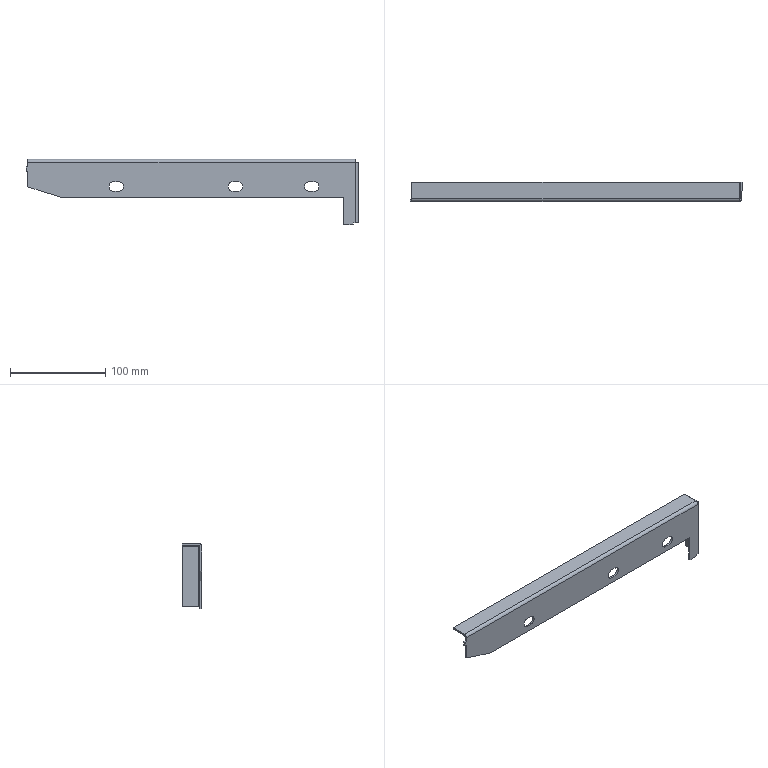Part | 1 solid | 43 faces | box 348 x 20 x 68.5 mm | volume 41297 mm3 | plane 33 | cylinder 10 | commonest cylinder face diameters 10 x6 2 x2 6 x2
STEP:
#1=CARTESIAN_POINT('',(-343.,-2.,53.5));
#2=VERTEX_POINT('',#1);
#3=CARTESIAN_POINT('',(-343.,-2.,37.5));
#4=VERTEX_POINT('',#3);
#5=CARTESIAN_POINT('',(-343.,-2.,63.5));
#6=DIRECTION('',(0.,0.,-1.));
#7=VECTOR('',#6,1000.);
#8=LINE('',#5,#7);
#9=EDGE_CURVE('',#2,#4,#8,.T.);
#10=ORIENTED_EDGE('',*,*,#9,.F.);
#11=CARTESIAN_POINT('',(-343.,0.,53.5));
#12=VERTEX_POINT('',#11);
#13=CARTESIAN_POINT('',(-343.,0.,53.5));
#14=DIRECTION('',(0.,-1.,0.));
#15=VECTOR('',#14,1000.);
#16=LINE('',#13,#15);
#17=EDGE_CURVE('',#12,#2,#16,.T.);
#18=ORIENTED_EDGE('',*,*,#17,.F.);
#19=CARTESIAN_POINT('',(-343.,0.,37.5));
#20=VERTEX_POINT('',#19);
#21=CARTESIAN_POINT('',(-343.,0.,63.5));
#22=DIRECTION('',(0.,0.,-1.));
#23=VECTOR('',#22,1000.);
#24=LINE('',#21,#23);
#25=EDGE_CURVE('',#12,#20,#24,.T.);
#26=ORIENTED_EDGE('',*,*,#25,.T.);
#27=CARTESIAN_POINT('',(-343.,8.,37.5));
#28=DIRECTION('',(0.,-1.,0.));
#29=VECTOR('',#28,1000.);
#30=LINE('',#27,#29);
#31=EDGE_CURVE('',#20,#4,#30,.T.);
#32=ORIENTED_EDGE('',*,*,#31,.T.);
#33=EDGE_LOOP('',(#10,#18,#26,#32));
#34=FACE_OUTER_BOUND('',#33,.T.);
#35=CARTESIAN_POINT('',(-343.,-2.,63.5));
#36=DIRECTION('',(-1.,0.,0.));
#37=DIRECTION('',(0.,0.,1.));
#38=AXIS2_PLACEMENT_3D('',#35,#36,#37);
#39=PLANE('',#38);
#40=ADVANCED_FACE('',(#34),#39,.T.);
#41=CARTESIAN_POINT('',(-343.,0.,63.5));
#42=VERTEX_POINT('',#41);
#43=CARTESIAN_POINT('',(-343.,0.,58.5));
#44=VERTEX_POINT('',#43);
#45=CARTESIAN_POINT('',(-343.,0.,63.5));
#46=DIRECTION('',(0.,0.,-1.));
#47=VECTOR('',#46,1000.);
#48=LINE('',#45,#47);
#49=EDGE_CURVE('',#42,#44,#48,.T.);
#50=ORIENTED_EDGE('',*,*,#49,.T.);
#51=CARTESIAN_POINT('',(-343.,-2.,58.5));
#52=VERTEX_POINT('',#51);
#53=CARTESIAN_POINT('',(-343.,0.,58.5));
#54=DIRECTION('',(0.,1.,0.));
#55=VECTOR('',#54,1000.);
#56=LINE('',#53,#55);
#57=EDGE_CURVE('',#52,#44,#56,.T.);
#58=ORIENTED_EDGE('',*,*,#57,.F.);
#59=CARTESIAN_POINT('',(-343.,-2.,63.5));
#60=VERTEX_POINT('',#59);
#61=CARTESIAN_POINT('',(-343.,-2.,63.5));
#62=DIRECTION('',(0.,0.,-1.));
#63=VECTOR('',#62,1000.);
#64=LINE('',#61,#63);
#65=EDGE_CURVE('',#60,#52,#64,.T.);
#66=ORIENTED_EDGE('',*,*,#65,.F.);
#67=CARTESIAN_POINT('',(-343.,-2.,63.5));
#68=DIRECTION('',(0.,1.,0.));
#69=VECTOR('',#68,1000.);
#70=LINE('',#67,#69);
#71=EDGE_CURVE('',#60,#42,#70,.T.);
#72=ORIENTED_EDGE('',*,*,#71,.T.);
#73=EDGE_LOOP('',(#50,#58,#66,#72));
#74=FACE_OUTER_BOUND('',#73,.T.);
#75=CARTESIAN_POINT('',(-343.,-2.,63.5));
#76=DIRECTION('',(-1.,0.,0.));
#77=DIRECTION('',(0.,0.,1.));
#78=AXIS2_PLACEMENT_3D('',#75,#76,#77);
#79=PLANE('',#78);
#80=ADVANCED_FACE('',(#74),#79,.T.);
#81=CARTESIAN_POINT('',(-253.,-2.,33.));
#82=VERTEX_POINT('',#81);
#83=CARTESIAN_POINT('',(-248.,-2.,33.));
#84=VERTEX_POINT('',#83);
#85=CARTESIAN_POINT('',(-253.,-2.,33.));
#86=DIRECTION('',(1.,0.,0.));
#87=VECTOR('',#86,1000.);
#88=LINE('',#85,#87);
#89=EDGE_CURVE('',#82,#84,#88,.T.);
#90=ORIENTED_EDGE('',*,*,#89,.F.);
#91=CARTESIAN_POINT('',(-253.,-2.,43.));
#92=VERTEX_POINT('',#91);
#93=CARTESIAN_POINT('',(-253.,-2.,38.));
#94=DIRECTION('',(0.,-1.,0.));
#95=DIRECTION('',(0.,0.,-1.));
#96=AXIS2_PLACEMENT_3D('',#93,#94,#95);
#97=CIRCLE('',#96,5.);
#98=EDGE_CURVE('',#92,#82,#97,.T.);
#99=ORIENTED_EDGE('',*,*,#98,.F.);
#100=CARTESIAN_POINT('',(-248.,-2.,43.));
#101=VERTEX_POINT('',#100);
#102=CARTESIAN_POINT('',(-253.,-2.,43.));
#103=DIRECTION('',(-1.,0.,0.));
#104=VECTOR('',#103,1000.);
#105=LINE('',#102,#104);
#106=EDGE_CURVE('',#101,#92,#105,.T.);
#107=ORIENTED_EDGE('',*,*,#106,.F.);
#108=CARTESIAN_POINT('',(-248.,-2.,38.));
#109=DIRECTION('',(0.,-1.,0.));
#110=DIRECTION('',(0.,0.,-1.));
#111=AXIS2_PLACEMENT_3D('',#108,#109,#110);
#112=CIRCLE('',#111,5.);
#113=EDGE_CURVE('',#84,#101,#112,.T.);
#114=ORIENTED_EDGE('',*,*,#113,.F.);
#115=EDGE_LOOP('',(#90,#99,#107,#114));
#116=FACE_BOUND('',#115,.T.);
#117=CARTESIAN_POINT('',(-128.,-2.,33.));
#118=VERTEX_POINT('',#117);
#119=CARTESIAN_POINT('',(-123.,-2.,33.));
#120=VERTEX_POINT('',#119);
#121=CARTESIAN_POINT('',(-128.,-2.,33.));
#122=DIRECTION('',(1.,0.,0.));
#123=VECTOR('',#122,1000.);
#124=LINE('',#121,#123);
#125=EDGE_CURVE('',#118,#120,#124,.T.);
#126=ORIENTED_EDGE('',*,*,#125,.F.);
#127=CARTESIAN_POINT('',(-128.,-2.,43.));
#128=VERTEX_POINT('',#127);
#129=CARTESIAN_POINT('',(-128.,-2.,38.));
#130=DIRECTION('',(0.,-1.,0.));
#131=DIRECTION('',(0.,0.,-1.));
#132=AXIS2_PLACEMENT_3D('',#129,#130,#131);
#133=CIRCLE('',#132,5.);
#134=EDGE_CURVE('',#128,#118,#133,.T.);
#135=ORIENTED_EDGE('',*,*,#134,.F.);
#136=CARTESIAN_POINT('',(-123.,-2.,43.));
#137=VERTEX_POINT('',#136);
#138=CARTESIAN_POINT('',(-128.,-2.,43.));
#139=DIRECTION('',(-1.,0.,0.));
#140=VECTOR('',#139,1000.);
#141=LINE('',#138,#140);
#142=EDGE_CURVE('',#137,#128,#141,.T.);
#143=ORIENTED_EDGE('',*,*,#142,.F.);
#144=CARTESIAN_POINT('',(-123.,-2.,38.));
#145=DIRECTION('',(0.,-1.,0.));
#146=DIRECTION('',(0.,0.,-1.));
#147=AXIS2_PLACEMENT_3D('',#144,#145,#146);
#148=CIRCLE('',#147,5.);
#149=EDGE_CURVE('',#120,#137,#148,.T.);
#150=ORIENTED_EDGE('',*,*,#149,.F.);
#151=EDGE_LOOP('',(#126,#135,#143,#150));
#152=FACE_BOUND('',#151,.T.);
#153=CARTESIAN_POINT('',(-48.,-2.,33.));
#154=VERTEX_POINT('',#153);
#155=CARTESIAN_POINT('',(-43.,-2.,33.));
#156=VERTEX_POINT('',#155);
#157=CARTESIAN_POINT('',(-48.,-2.,33.));
#158=DIRECTION('',(1.,0.,0.));
#159=VECTOR('',#158,1000.);
#160=LINE('',#157,#159);
#161=EDGE_CURVE('',#154,#156,#160,.T.);
#162=ORIENTED_EDGE('',*,*,#161,.F.);
#163=CARTESIAN_POINT('',(-48.,-2.,43.));
#164=VERTEX_POINT('',#163);
#165=CARTESIAN_POINT('',(-48.,-2.,38.));
#166=DIRECTION('',(0.,-1.,0.));
#167=DIRECTION('',(0.,0.,-1.));
#168=AXIS2_PLACEMENT_3D('',#165,#166,#167);
#169=CIRCLE('',#168,5.);
#170=EDGE_CURVE('',#164,#154,#169,.T.);
#171=ORIENTED_EDGE('',*,*,#170,.F.);
#172=CARTESIAN_POINT('',(-43.,-2.,43.));
#173=VERTEX_POINT('',#172);
#174=CARTESIAN_POINT('',(-48.,-2.,43.));
#175=DIRECTION('',(-1.,0.,0.));
#176=VECTOR('',#175,1000.);
#177=LINE('',#174,#176);
#178=EDGE_CURVE('',#173,#164,#177,.T.);
#179=ORIENTED_EDGE('',*,*,#178,.F.);
#180=CARTESIAN_POINT('',(-43.,-2.,38.));
#181=DIRECTION('',(0.,-1.,0.));
#182=DIRECTION('',(0.,0.,-1.));
#183=AXIS2_PLACEMENT_3D('',#180,#181,#182);
#184=CIRCLE('',#183,5.);
#185=EDGE_CURVE('',#156,#173,#184,.T.);
#186=ORIENTED_EDGE('',*,*,#185,.F.);
#187=EDGE_LOOP('',(#162,#171,#179,#186));
#188=FACE_BOUND('',#187,.T.);
#189=ORIENTED_EDGE('',*,*,#65,.T.);
#190=CARTESIAN_POINT('',(-345.,-2.,58.5));
#191=VERTEX_POINT('',#190);
#192=CARTESIAN_POINT('',(-345.,-2.,58.5));
#193=DIRECTION('',(1.,0.,0.));
#194=VECTOR('',#193,1000.);
#195=LINE('',#192,#194);
#196=EDGE_CURVE('',#191,#52,#195,.T.);
#197=ORIENTED_EDGE('',*,*,#196,.F.);
#198=CARTESIAN_POINT('',(-345.,-2.,53.5));
#199=VERTEX_POINT('',#198);
#200=CARTESIAN_POINT('',(-345.,-2.,53.5));
#201=DIRECTION('',(0.,0.,1.));
#202=VECTOR('',#201,1000.);
#203=LINE('',#200,#202);
#204=EDGE_CURVE('',#199,#191,#203,.T.);
#205=ORIENTED_EDGE('',*,*,#204,.F.);
#206=CARTESIAN_POINT('',(-345.,-2.,53.5));
#207=DIRECTION('',(1.,0.,0.));
#208=VECTOR('',#207,1000.);
#209=LINE('',#206,#208);
#210=EDGE_CURVE('',#199,#2,#209,.T.);
#211=ORIENTED_EDGE('',*,*,#210,.T.);
#212=ORIENTED_EDGE('',*,*,#9,.T.);
#213=CARTESIAN_POINT('',(-308.,-2.,26.5));
#214=VERTEX_POINT('',#213);
#215=CARTESIAN_POINT('',(-343.,-2.,37.5));
#216=DIRECTION('',(-0.954,0.,0.2998));
#217=VECTOR('',#216,1000.);
#218=LINE('',#215,#217);
#219=EDGE_CURVE('',#214,#4,#218,.T.);
#220=ORIENTED_EDGE('',*,*,#219,.F.);
#221=CARTESIAN_POINT('',(-12.,-2.,26.5));
#222=VERTEX_POINT('',#221);
#223=CARTESIAN_POINT('',(-343.,-2.,26.5));
#224=DIRECTION('',(-1.,0.,0.));
#225=VECTOR('',#224,1000.);
#226=LINE('',#223,#225);
#227=EDGE_CURVE('',#222,#214,#226,.T.);
#228=ORIENTED_EDGE('',*,*,#227,.F.);
#229=CARTESIAN_POINT('',(-12.,-2.,-2.));
#230=VERTEX_POINT('',#229);
#231=CARTESIAN_POINT('',(-12.,-2.,0.));
#232=DIRECTION('',(0.,0.,1.));
#233=VECTOR('',#232,1000.);
#234=LINE('',#231,#233);
#235=EDGE_CURVE('',#230,#222,#234,.T.);
#236=ORIENTED_EDGE('',*,*,#235,.F.);
#237=CARTESIAN_POINT('',(-2.,-2.,-2.));
#238=VERTEX_POINT('',#237);
#239=CARTESIAN_POINT('',(-12.,-2.,-2.));
#240=DIRECTION('',(1.,0.,0.));
#241=VECTOR('',#240,1000.);
#242=LINE('',#239,#241);
#243=EDGE_CURVE('',#230,#238,#242,.T.);
#244=ORIENTED_EDGE('',*,*,#243,.T.);
#245=CARTESIAN_POINT('',(-2.,-2.,0.));
#246=VERTEX_POINT('',#245);
#247=CARTESIAN_POINT('',(-2.,-2.,0.));
#248=DIRECTION('',(0.,0.,1.));
#249=VECTOR('',#248,1000.);
#250=LINE('',#247,#249);
#251=EDGE_CURVE('',#238,#246,#250,.T.);
#252=ORIENTED_EDGE('',*,*,#251,.T.);
#253=CARTESIAN_POINT('',(0.,-2.,0.));
#254=VERTEX_POINT('',#253);
#255=CARTESIAN_POINT('',(-343.,-2.,0.));
#256=DIRECTION('',(1.,0.,0.));
#257=VECTOR('',#256,1000.);
#258=LINE('',#255,#257);
#259=EDGE_CURVE('',#246,#254,#258,.T.);
#260=ORIENTED_EDGE('',*,*,#259,.T.);
#261=CARTESIAN_POINT('',(0.,-2.,63.5));
#262=VERTEX_POINT('',#261);
#263=CARTESIAN_POINT('',(0.,-2.,63.5));
#264=DIRECTION('',(0.,0.,-1.));
#265=VECTOR('',#264,1000.);
#266=LINE('',#263,#265);
#267=EDGE_CURVE('',#262,#254,#266,.T.);
#268=ORIENTED_EDGE('',*,*,#267,.F.);
#269=CARTESIAN_POINT('',(-343.,-2.,63.5));
#270=DIRECTION('',(1.,0.,0.));
#271=VECTOR('',#270,1000.);
#272=LINE('',#269,#271);
#273=EDGE_CURVE('',#60,#262,#272,.T.);
#274=ORIENTED_EDGE('',*,*,#273,.F.);
#275=EDGE_LOOP('',(#189,#197,#205,#211,#212,#220,#228,#236,#244,#252,#260,#268,#274));
#276=FACE_OUTER_BOUND('',#275,.T.);
#277=CARTESIAN_POINT('',(-343.,-2.,63.5));
#278=DIRECTION('',(0.,1.,0.));
#279=DIRECTION('',(0.,0.,1.));
#280=AXIS2_PLACEMENT_3D('',#277,#278,#279);
#281=PLANE('',#280);
#282=ADVANCED_FACE('',(#116,#152,#188,#276),#281,.F.);
#283=CARTESIAN_POINT('',(-308.,0.,26.5));
#284=VERTEX_POINT('',#283);
#285=CARTESIAN_POINT('',(-350.437,0.,39.837));
#286=DIRECTION('',(0.954,0.,-0.2998));
#287=VECTOR('',#286,1000.);
#288=LINE('',#285,#287);
#289=EDGE_CURVE('',#20,#284,#288,.T.);
#290=ORIENTED_EDGE('',*,*,#289,.F.);
#291=ORIENTED_EDGE('',*,*,#25,.F.);
#292=CARTESIAN_POINT('',(-345.,0.,53.5));
#293=VERTEX_POINT('',#292);
#294=CARTESIAN_POINT('',(-345.,0.,53.5));
#295=DIRECTION('',(1.,0.,0.));
#296=VECTOR('',#295,1000.);
#297=LINE('',#294,#296);
#298=EDGE_CURVE('',#293,#12,#297,.T.);
#299=ORIENTED_EDGE('',*,*,#298,.F.);
#300=CARTESIAN_POINT('',(-345.,0.,58.5));
#301=VERTEX_POINT('',#300);
#302=CARTESIAN_POINT('',(-345.,0.,53.5));
#303=DIRECTION('',(0.,0.,-1.));
#304=VECTOR('',#303,1000.);
#305=LINE('',#302,#304);
#306=EDGE_CURVE('',#301,#293,#305,.T.);
#307=ORIENTED_EDGE('',*,*,#306,.F.);
#308=CARTESIAN_POINT('',(-345.,0.,58.5));
#309=DIRECTION('',(1.,0.,0.));
#310=VECTOR('',#309,1000.);
#311=LINE('',#308,#310);
#312=EDGE_CURVE('',#301,#44,#311,.T.);
#313=ORIENTED_EDGE('',*,*,#312,.T.);
#314=ORIENTED_EDGE('',*,*,#49,.F.);
#315=CARTESIAN_POINT('',(0.,0.,63.5));
#316=VERTEX_POINT('',#315);
#317=CARTESIAN_POINT('',(-343.,0.,63.5));
#318=DIRECTION('',(1.,0.,0.));
#319=VECTOR('',#318,1000.);
#320=LINE('',#317,#319);
#321=EDGE_CURVE('',#42,#316,#320,.T.);
#322=ORIENTED_EDGE('',*,*,#321,.T.);
#323=CARTESIAN_POINT('',(0.,0.,0.));
#324=VERTEX_POINT('',#323);
#325=CARTESIAN_POINT('',(0.,0.,63.5));
#326=DIRECTION('',(0.,0.,-1.));
#327=VECTOR('',#326,1000.);
#328=LINE('',#325,#327);
#329=EDGE_CURVE('',#316,#324,#328,.T.);
#330=ORIENTED_EDGE('',*,*,#329,.T.);
#331=CARTESIAN_POINT('',(-2.,0.,0.));
#332=VERTEX_POINT('',#331);
#333=CARTESIAN_POINT('',(-343.,0.,0.));
#334=DIRECTION('',(1.,0.,0.));
#335=VECTOR('',#334,1000.);
#336=LINE('',#333,#335);
#337=EDGE_CURVE('',#332,#324,#336,.T.);
#338=ORIENTED_EDGE('',*,*,#337,.F.);
#339=CARTESIAN_POINT('',(-2.,0.,-2.));
#340=VERTEX_POINT('',#339);
#341=CARTESIAN_POINT('',(-2.,0.,0.));
#342=DIRECTION('',(0.,0.,1.));
#343=VECTOR('',#342,1000.);
#344=LINE('',#341,#343);
#345=EDGE_CURVE('',#340,#332,#344,.T.);
#346=ORIENTED_EDGE('',*,*,#345,.F.);
#347=CARTESIAN_POINT('',(-12.,0.,-2.));
#348=VERTEX_POINT('',#347);
#349=CARTESIAN_POINT('',(-12.,0.,-2.));
#350=DIRECTION('',(1.,0.,0.));
#351=VECTOR('',#350,1000.);
#352=LINE('',#349,#351);
#353=EDGE_CURVE('',#348,#340,#352,.T.);
#354=ORIENTED_EDGE('',*,*,#353,.F.);
#355=CARTESIAN_POINT('',(-12.,0.,26.5));
#356=VERTEX_POINT('',#355);
#357=CARTESIAN_POINT('',(-12.,0.,63.5));
#358=DIRECTION('',(0.,0.,-1.));
#359=VECTOR('',#358,1000.);
#360=LINE('',#357,#359);
#361=EDGE_CURVE('',#356,#348,#360,.T.);
#362=ORIENTED_EDGE('',*,*,#361,.F.);
#363=CARTESIAN_POINT('',(-343.,0.,26.5));
#364=DIRECTION('',(1.,0.,0.));
#365=VECTOR('',#364,1000.);
#366=LINE('',#363,#365);
#367=EDGE_CURVE('',#284,#356,#366,.T.);
#368=ORIENTED_EDGE('',*,*,#367,.F.);
#369=EDGE_LOOP('',(#290,#291,#299,#307,#313,#314,#322,#330,#338,#346,#354,#362,#368));
#370=FACE_OUTER_BOUND('',#369,.T.);
#371=CARTESIAN_POINT('',(-253.,0.,33.));
#372=VERTEX_POINT('',#371);
#373=CARTESIAN_POINT('',(-253.,0.,43.));
#374=VERTEX_POINT('',#373);
#375=CARTESIAN_POINT('',(-253.,0.,38.));
#376=DIRECTION('',(0.,1.,0.));
#377=DIRECTION('',(0.,0.,1.));
#378=AXIS2_PLACEMENT_3D('',#375,#376,#377);
#379=CIRCLE('',#378,5.);
#380=EDGE_CURVE('',#372,#374,#379,.T.);
#381=ORIENTED_EDGE('',*,*,#380,.F.);
#382=CARTESIAN_POINT('',(-248.,0.,33.));
#383=VERTEX_POINT('',#382);
#384=CARTESIAN_POINT('',(-343.,0.,33.));
#385=DIRECTION('',(-1.,0.,0.));
#386=VECTOR('',#385,1000.);
#387=LINE('',#384,#386);
#388=EDGE_CURVE('',#383,#372,#387,.T.);
#389=ORIENTED_EDGE('',*,*,#388,.F.);
#390=CARTESIAN_POINT('',(-248.,0.,43.));
#391=VERTEX_POINT('',#390);
#392=CARTESIAN_POINT('',(-248.,0.,38.));
#393=DIRECTION('',(0.,1.,0.));
#394=DIRECTION('',(0.,0.,1.));
#395=AXIS2_PLACEMENT_3D('',#392,#393,#394);
#396=CIRCLE('',#395,5.);
#397=EDGE_CURVE('',#391,#383,#396,.T.);
#398=ORIENTED_EDGE('',*,*,#397,.F.);
#399=CARTESIAN_POINT('',(-343.,0.,43.));
#400=DIRECTION('',(1.,0.,0.));
#401=VECTOR('',#400,1000.);
#402=LINE('',#399,#401);
#403=EDGE_CURVE('',#374,#391,#402,.T.);
#404=ORIENTED_EDGE('',*,*,#403,.F.);
#405=EDGE_LOOP('',(#381,#389,#398,#404));
#406=FACE_BOUND('',#405,.T.);
#407=CARTESIAN_POINT('',(-128.,0.,33.));
#408=VERTEX_POINT('',#407);
#409=CARTESIAN_POINT('',(-128.,0.,43.));
#410=VERTEX_POINT('',#409);
#411=CARTESIAN_POINT('',(-128.,0.,38.));
#412=DIRECTION('',(0.,1.,0.));
#413=DIRECTION('',(0.,0.,1.));
#414=AXIS2_PLACEMENT_3D('',#411,#412,#413);
#415=CIRCLE('',#414,5.);
#416=EDGE_CURVE('',#408,#410,#415,.T.);
#417=ORIENTED_EDGE('',*,*,#416,.F.);
#418=CARTESIAN_POINT('',(-123.,0.,33.));
#419=VERTEX_POINT('',#418);
#420=CARTESIAN_POINT('',(-343.,0.,33.));
#421=DIRECTION('',(-1.,0.,0.));
#422=VECTOR('',#421,1000.);
#423=LINE('',#420,#422);
#424=EDGE_CURVE('',#419,#408,#423,.T.);
#425=ORIENTED_EDGE('',*,*,#424,.F.);
#426=CARTESIAN_POINT('',(-123.,0.,43.));
#427=VERTEX_POINT('',#426);
#428=CARTESIAN_POINT('',(-123.,0.,38.));
#429=DIRECTION('',(0.,1.,0.));
#430=DIRECTION('',(0.,0.,1.));
#431=AXIS2_PLACEMENT_3D('',#428,#429,#430);
#432=CIRCLE('',#431,5.);
#433=EDGE_CURVE('',#427,#419,#432,.T.);
#434=ORIENTED_EDGE('',*,*,#433,.F.);
#435=CARTESIAN_POINT('',(-343.,0.,43.));
#436=DIRECTION('',(1.,0.,0.));
#437=VECTOR('',#436,1000.);
#438=LINE('',#435,#437);
#439=EDGE_CURVE('',#410,#427,#438,.T.);
#440=ORIENTED_EDGE('',*,*,#439,.F.);
#441=EDGE_LOOP('',(#417,#425,#434,#440));
#442=FACE_BOUND('',#441,.T.);
#443=CARTESIAN_POINT('',(-48.,0.,33.));
#444=VERTEX_POINT('',#443);
#445=CARTESIAN_POINT('',(-48.,0.,43.));
#446=VERTEX_POINT('',#445);
#447=CARTESIAN_POINT('',(-48.,0.,38.));
#448=DIRECTION('',(0.,1.,0.));
#449=DIRECTION('',(0.,0.,1.));
#450=AXIS2_PLACEMENT_3D('',#447,#448,#449);
#451=CIRCLE('',#450,5.);
#452=EDGE_CURVE('',#444,#446,#451,.T.);
#453=ORIENTED_EDGE('',*,*,#452,.F.);
#454=CARTESIAN_POINT('',(-43.,0.,33.));
#455=VERTEX_POINT('',#454);
#456=CARTESIAN_POINT('',(-343.,0.,33.));
#457=DIRECTION('',(-1.,0.,0.));
#458=VECTOR('',#457,1000.);
#459=LINE('',#456,#458);
#460=EDGE_CURVE('',#455,#444,#459,.T.);
#461=ORIENTED_EDGE('',*,*,#460,.F.);
#462=CARTESIAN_POINT('',(-43.,0.,43.));
#463=VERTEX_POINT('',#462);
#464=CARTESIAN_POINT('',(-43.,0.,38.));
#465=DIRECTION('',(0.,1.,0.));
#466=DIRECTION('',(0.,0.,1.));
#467=AXIS2_PLACEMENT_3D('',#464,#465,#466);
#468=CIRCLE('',#467,5.);
#469=EDGE_CURVE('',#463,#455,#468,.T.);
#470=ORIENTED_EDGE('',*,*,#469,.F.);
#471=CARTESIAN_POINT('',(-343.,0.,43.));
#472=DIRECTION('',(1.,0.,0.));
#473=VECTOR('',#472,1000.);
#474=LINE('',#471,#473);
#475=EDGE_CURVE('',#446,#463,#474,.T.);
#476=ORIENTED_EDGE('',*,*,#475,.F.);
#477=EDGE_LOOP('',(#453,#461,#470,#476));
#478=FACE_BOUND('',#477,.T.);
#479=CARTESIAN_POINT('',(-343.,0.,63.5));
#480=DIRECTION('',(0.,1.,0.));
#481=DIRECTION('',(0.,0.,1.));
#482=AXIS2_PLACEMENT_3D('',#479,#480,#481);
#483=PLANE('',#482);
#484=ADVANCED_FACE('',(#370,#406,#442,#478),#483,.T.);
#485=CARTESIAN_POINT('',(-2.,0.,0.));
#486=DIRECTION('',(0.,-1.,0.));
#487=VECTOR('',#486,1000.);
#488=LINE('',#485,#487);
#489=EDGE_CURVE('',#332,#246,#488,.T.);
#490=ORIENTED_EDGE('',*,*,#489,.F.);
#491=ORIENTED_EDGE('',*,*,#337,.T.);
#492=CARTESIAN_POINT('',(0.,0.,0.));
#493=DIRECTION('',(0.,-1.,0.));
#494=VECTOR('',#493,1000.);
#495=LINE('',#492,#494);
#496=EDGE_CURVE('',#324,#254,#495,.T.);
#497=ORIENTED_EDGE('',*,*,#496,.T.);
#498=ORIENTED_EDGE('',*,*,#259,.F.);
#499=EDGE_LOOP('',(#490,#491,#497,#498));
#500=FACE_OUTER_BOUND('',#499,.T.);
#501=CARTESIAN_POINT('',(0.,0.,0.));
#502=DIRECTION('',(0.,0.,-1.));
#503=DIRECTION('',(-1.,0.,0.));
#504=AXIS2_PLACEMENT_3D('',#501,#502,#503);
#505=PLANE('',#504);
#506=ADVANCED_FACE('',(#500),#505,.T.);
#507=CARTESIAN_POINT('',(-343.,1.,64.5));
#508=VERTEX_POINT('',#507);
#509=CARTESIAN_POINT('',(-343.,1.,66.5));
#510=VERTEX_POINT('',#509);
#511=CARTESIAN_POINT('',(-343.,1.,66.5));
#512=DIRECTION('',(0.,0.,1.));
#513=VECTOR('',#512,1000.);
#514=LINE('',#511,#513);
#515=EDGE_CURVE('',#508,#510,#514,.T.);
#516=ORIENTED_EDGE('',*,*,#515,.F.);
#517=CARTESIAN_POINT('',(-343.,1.,63.5));
#518=DIRECTION('',(-1.,0.,0.));
#519=DIRECTION('',(0.,0.,-1.));
#520=AXIS2_PLACEMENT_3D('',#517,#518,#519);
#521=CIRCLE('',#520,1.);
#522=EDGE_CURVE('',#42,#508,#521,.T.);
#523=ORIENTED_EDGE('',*,*,#522,.F.);
#524=ORIENTED_EDGE('',*,*,#71,.F.);
#525=CARTESIAN_POINT('',(-343.,1.,63.5));
#526=DIRECTION('',(-1.,0.,0.));
#527=DIRECTION('',(0.,0.,-1.));
#528=AXIS2_PLACEMENT_3D('',#525,#526,#527);
#529=CIRCLE('',#528,3.);
#530=EDGE_CURVE('',#60,#510,#529,.T.);
#531=ORIENTED_EDGE('',*,*,#530,.T.);
#532=EDGE_LOOP('',(#516,#523,#524,#531));
#533=FACE_OUTER_BOUND('',#532,.T.);
#534=CARTESIAN_POINT('',(-343.,1.,63.5));
#535=DIRECTION('',(-1.,0.,0.));
#536=DIRECTION('',(0.,0.,1.));
#537=AXIS2_PLACEMENT_3D('',#534,#535,#536);
#538=PLANE('',#537);
#539=ADVANCED_FACE('',(#533),#538,.T.);
#540=CARTESIAN_POINT('',(0.,1.,64.5));
#541=VERTEX_POINT('',#540);
#542=CARTESIAN_POINT('',(0.,1.,63.5));
#543=DIRECTION('',(1.,0.,0.));
#544=DIRECTION('',(0.,0.,-1.));
#545=AXIS2_PLACEMENT_3D('',#542,#543,#544);
#546=CIRCLE('',#545,1.);
#547=EDGE_CURVE('',#541,#316,#546,.T.);
#548=ORIENTED_EDGE('',*,*,#547,.F.);
#549=CARTESIAN_POINT('',(0.,1.,66.5));
#550=VERTEX_POINT('',#549);
#551=CARTESIAN_POINT('',(0.,1.,64.5));
#552=DIRECTION('',(0.,0.,1.));
#553=VECTOR('',#552,1000.);
#554=LINE('',#551,#553);
#555=EDGE_CURVE('',#541,#550,#554,.T.);
#556=ORIENTED_EDGE('',*,*,#555,.T.);
#557=CARTESIAN_POINT('',(0.,1.,63.5));
#558=DIRECTION('',(1.,0.,0.));
#559=DIRECTION('',(0.,0.,-1.));
#560=AXIS2_PLACEMENT_3D('',#557,#558,#559);
#561=CIRCLE('',#560,3.);
#562=EDGE_CURVE('',#550,#262,#561,.T.);
#563=ORIENTED_EDGE('',*,*,#562,.T.);
#564=CARTESIAN_POINT('',(0.,0.,63.5));
#565=DIRECTION('',(0.,-1.,0.));
#566=VECTOR('',#565,1000.);
#567=LINE('',#564,#566);
#568=EDGE_CURVE('',#316,#262,#567,.T.);
#569=ORIENTED_EDGE('',*,*,#568,.F.);
#570=EDGE_LOOP('',(#548,#556,#563,#569));
#571=FACE_OUTER_BOUND('',#570,.T.);
#572=CARTESIAN_POINT('',(0.,1.,63.5));
#573=DIRECTION('',(-1.,0.,0.));
#574=DIRECTION('',(0.,0.,1.));
#575=AXIS2_PLACEMENT_3D('',#572,#573,#574);
#576=PLANE('',#575);
#577=ADVANCED_FACE('',(#571),#576,.F.);
#578=ORIENTED_EDGE('',*,*,#273,.T.);
#579=ORIENTED_EDGE('',*,*,#562,.F.);
#580=CARTESIAN_POINT('',(-343.,1.,66.5));
#581=DIRECTION('',(-1.,0.,0.));
#582=VECTOR('',#581,1000.);
#583=LINE('',#580,#582);
#584=EDGE_CURVE('',#550,#510,#583,.T.);
#585=ORIENTED_EDGE('',*,*,#584,.T.);
#586=ORIENTED_EDGE('',*,*,#530,.F.);
#587=EDGE_LOOP('',(#578,#579,#585,#586));
#588=FACE_OUTER_BOUND('',#587,.T.);
#589=CARTESIAN_POINT('',(0.,1.,63.5));
#590=DIRECTION('',(1.,0.,0.));
#591=DIRECTION('',(0.,0.,1.));
#592=AXIS2_PLACEMENT_3D('',#589,#590,#591);
#593=CYLINDRICAL_SURFACE('',#592,3.);
#594=ADVANCED_FACE('',(#588),#593,.T.);
#595=ORIENTED_EDGE('',*,*,#321,.F.);
#596=ORIENTED_EDGE('',*,*,#522,.T.);
#597=CARTESIAN_POINT('',(-343.,1.,64.5));
#598=DIRECTION('',(1.,0.,0.));
#599=VECTOR('',#598,1000.);
#600=LINE('',#597,#599);
#601=EDGE_CURVE('',#508,#541,#600,.T.);
#602=ORIENTED_EDGE('',*,*,#601,.T.);
#603=ORIENTED_EDGE('',*,*,#547,.T.);
#604=EDGE_LOOP('',(#595,#596,#602,#603));
#605=FACE_OUTER_BOUND('',#604,.T.);
#606=CARTESIAN_POINT('',(0.,1.,63.5));
#607=DIRECTION('',(1.,0.,0.));
#608=DIRECTION('',(0.,0.,1.));
#609=AXIS2_PLACEMENT_3D('',#606,#607,#608);
#610=CYLINDRICAL_SURFACE('',#609,1.);
#611=ADVANCED_FACE('',(#605),#610,.F.);
#612=ORIENTED_EDGE('',*,*,#515,.T.);
#613=CARTESIAN_POINT('',(-343.,18.,66.5));
#614=VERTEX_POINT('',#613);
#615=CARTESIAN_POINT('',(-343.,0.,66.5));
#616=DIRECTION('',(0.,-1.,0.));
#617=VECTOR('',#616,1000.);
#618=LINE('',#615,#617);
#619=EDGE_CURVE('',#614,#510,#618,.T.);
#620=ORIENTED_EDGE('',*,*,#619,.F.);
#621=CARTESIAN_POINT('',(-343.,18.,64.5));
#622=VERTEX_POINT('',#621);
#623=CARTESIAN_POINT('',(-343.,18.,66.5));
#624=DIRECTION('',(0.,0.,-1.));
#625=VECTOR('',#624,1000.);
#626=LINE('',#623,#625);
#627=EDGE_CURVE('',#614,#622,#626,.T.);
#628=ORIENTED_EDGE('',*,*,#627,.T.);
#629=CARTESIAN_POINT('',(-343.,0.,64.5));
#630=DIRECTION('',(0.,-1.,0.));
#631=VECTOR('',#630,1000.);
#632=LINE('',#629,#631);
#633=EDGE_CURVE('',#622,#508,#632,.T.);
#634=ORIENTED_EDGE('',*,*,#633,.T.);
#635=EDGE_LOOP('',(#612,#620,#628,#634));
#636=FACE_OUTER_BOUND('',#635,.T.);
#637=CARTESIAN_POINT('',(-343.,0.,66.5));
#638=DIRECTION('',(1.,0.,0.));
#639=DIRECTION('',(0.,0.,-1.));
#640=AXIS2_PLACEMENT_3D('',#637,#638,#639);
#641=PLANE('',#640);
#642=ADVANCED_FACE('',(#636),#641,.F.);
#643=ORIENTED_EDGE('',*,*,#555,.F.);
#644=CARTESIAN_POINT('',(0.,18.,64.5));
#645=VERTEX_POINT('',#644);
#646=CARTESIAN_POINT('',(0.,18.,64.5));
#647=DIRECTION('',(0.,1.,0.));
#648=VECTOR('',#647,1000.);
#649=LINE('',#646,#648);
#650=EDGE_CURVE('',#541,#645,#649,.T.);
#651=ORIENTED_EDGE('',*,*,#650,.T.);
#652=CARTESIAN_POINT('',(0.,18.,66.5));
#653=VERTEX_POINT('',#652);
#654=CARTESIAN_POINT('',(0.,18.,66.5));
#655=DIRECTION('',(0.,0.,-1.));
#656=VECTOR('',#655,1000.);
#657=LINE('',#654,#656);
#658=EDGE_CURVE('',#653,#645,#657,.T.);
#659=ORIENTED_EDGE('',*,*,#658,.F.);
#660=CARTESIAN_POINT('',(0.,0.,66.5));
#661=DIRECTION('',(0.,1.,0.));
#662=VECTOR('',#661,1000.);
#663=LINE('',#660,#662);
#664=EDGE_CURVE('',#550,#653,#663,.T.);
#665=ORIENTED_EDGE('',*,*,#664,.F.);
#666=EDGE_LOOP('',(#643,#651,#659,#665));
#667=FACE_OUTER_BOUND('',#666,.T.);
#668=CARTESIAN_POINT('',(0.,18.,66.5));
#669=DIRECTION('',(-1.,0.,0.));
#670=DIRECTION('',(0.,0.,1.));
#671=AXIS2_PLACEMENT_3D('',#668,#669,#670);
#672=PLANE('',#671);
#673=ADVANCED_FACE('',(#667),#672,.F.);
#674=ORIENTED_EDGE('',*,*,#584,.F.);
#675=ORIENTED_EDGE('',*,*,#664,.T.);
#676=CARTESIAN_POINT('',(0.,18.,66.5));
#677=DIRECTION('',(-1.,0.,0.));
#678=VECTOR('',#677,1000.);
#679=LINE('',#676,#678);
#680=EDGE_CURVE('',#653,#614,#679,.T.);
#681=ORIENTED_EDGE('',*,*,#680,.T.);
#682=ORIENTED_EDGE('',*,*,#619,.T.);
#683=EDGE_LOOP('',(#674,#675,#681,#682));
#684=FACE_OUTER_BOUND('',#683,.T.);
#685=CARTESIAN_POINT('',(0.,0.,66.5));
#686=DIRECTION('',(0.,0.,-1.));
#687=DIRECTION('',(-1.,0.,0.));
#688=AXIS2_PLACEMENT_3D('',#685,#686,#687);
#689=PLANE('',#688);
#690=ADVANCED_FACE('',(#684),#689,.F.);
#691=ORIENTED_EDGE('',*,*,#650,.F.);
#692=ORIENTED_EDGE('',*,*,#601,.F.);
#693=ORIENTED_EDGE('',*,*,#633,.F.);
#694=CARTESIAN_POINT('',(-343.,18.,64.5));
#695=DIRECTION('',(-1.,0.,0.));
#696=VECTOR('',#695,1000.);
#697=LINE('',#694,#696);
#698=EDGE_CURVE('',#645,#622,#697,.T.);
#699=ORIENTED_EDGE('',*,*,#698,.F.);
#700=EDGE_LOOP('',(#691,#692,#693,#699));
#701=FACE_OUTER_BOUND('',#700,.T.);
#702=CARTESIAN_POINT('',(0.,0.,64.5));
#703=DIRECTION('',(0.,0.,-1.));
#704=DIRECTION('',(-1.,0.,0.));
#705=AXIS2_PLACEMENT_3D('',#702,#703,#704);
#706=PLANE('',#705);
#707=ADVANCED_FACE('',(#701),#706,.T.);
#708=ORIENTED_EDGE('',*,*,#698,.T.);
#709=ORIENTED_EDGE('',*,*,#627,.F.);
#710=ORIENTED_EDGE('',*,*,#680,.F.);
#711=ORIENTED_EDGE('',*,*,#658,.T.);
#712=EDGE_LOOP('',(#708,#709,#710,#711));
#713=FACE_OUTER_BOUND('',#712,.T.);
#714=CARTESIAN_POINT('',(-343.,18.,66.5));
#715=DIRECTION('',(0.,-1.,0.));
#716=DIRECTION('',(0.,0.,-1.));
#717=AXIS2_PLACEMENT_3D('',#714,#715,#716);
#718=PLANE('',#717);
#719=ADVANCED_FACE('',(#713),#718,.F.);
#720=CARTESIAN_POINT('',(1.,1.,63.5));
#721=VERTEX_POINT('',#720);
#722=CARTESIAN_POINT('',(3.,1.,63.5));
#723=VERTEX_POINT('',#722);
#724=CARTESIAN_POINT('',(3.,1.,63.5));
#725=DIRECTION('',(1.,0.,0.));
#726=VECTOR('',#725,1000.);
#727=LINE('',#724,#726);
#728=EDGE_CURVE('',#721,#723,#727,.T.);
#729=ORIENTED_EDGE('',*,*,#728,.F.);
#730=CARTESIAN_POINT('',(0.,1.,63.5));
#731=DIRECTION('',(0.,0.,1.));
#732=DIRECTION('',(-1.,0.,0.));
#733=AXIS2_PLACEMENT_3D('',#730,#731,#732);
#734=CIRCLE('',#733,1.);
#735=EDGE_CURVE('',#316,#721,#734,.T.);
#736=ORIENTED_EDGE('',*,*,#735,.F.);
#737=ORIENTED_EDGE('',*,*,#568,.T.);
#738=CARTESIAN_POINT('',(0.,1.,63.5));
#739=DIRECTION('',(0.,0.,1.));
#740=DIRECTION('',(-1.,0.,0.));
#741=AXIS2_PLACEMENT_3D('',#738,#739,#740);
#742=CIRCLE('',#741,3.);
#743=EDGE_CURVE('',#262,#723,#742,.T.);
#744=ORIENTED_EDGE('',*,*,#743,.T.);
#745=EDGE_LOOP('',(#729,#736,#737,#744));
#746=FACE_OUTER_BOUND('',#745,.T.);
#747=CARTESIAN_POINT('',(0.,1.,63.5));
#748=DIRECTION('',(0.,0.,1.));
#749=DIRECTION('',(1.,0.,0.));
#750=AXIS2_PLACEMENT_3D('',#747,#748,#749);
#751=PLANE('',#750);
#752=ADVANCED_FACE('',(#746),#751,.T.);
#753=CARTESIAN_POINT('',(1.,1.,0.));
#754=VERTEX_POINT('',#753);
#755=CARTESIAN_POINT('',(0.,1.,0.));
#756=DIRECTION('',(0.,0.,-1.));
#757=DIRECTION('',(-1.,0.,0.));
#758=AXIS2_PLACEMENT_3D('',#755,#756,#757);
#759=CIRCLE('',#758,1.);
#760=EDGE_CURVE('',#754,#324,#759,.T.);
#761=ORIENTED_EDGE('',*,*,#760,.F.);
#762=CARTESIAN_POINT('',(3.,1.,0.));
#763=VERTEX_POINT('',#762);
#764=CARTESIAN_POINT('',(1.,1.,0.));
#765=DIRECTION('',(1.,0.,0.));
#766=VECTOR('',#765,1000.);
#767=LINE('',#764,#766);
#768=EDGE_CURVE('',#754,#763,#767,.T.);
#769=ORIENTED_EDGE('',*,*,#768,.T.);
#770=CARTESIAN_POINT('',(0.,1.,0.));
#771=DIRECTION('',(0.,0.,-1.));
#772=DIRECTION('',(-1.,0.,0.));
#773=AXIS2_PLACEMENT_3D('',#770,#771,#772);
#774=CIRCLE('',#773,3.);
#775=EDGE_CURVE('',#763,#254,#774,.T.);
#776=ORIENTED_EDGE('',*,*,#775,.T.);
#777=ORIENTED_EDGE('',*,*,#496,.F.);
#778=EDGE_LOOP('',(#761,#769,#776,#777));
#779=FACE_OUTER_BOUND('',#778,.T.);
#780=CARTESIAN_POINT('',(0.,1.,0.));
#781=DIRECTION('',(0.,0.,1.));
#782=DIRECTION('',(1.,0.,0.));
#783=AXIS2_PLACEMENT_3D('',#780,#781,#782);
#784=PLANE('',#783);
#785=ADVANCED_FACE('',(#779),#784,.F.);
#786=ORIENTED_EDGE('',*,*,#267,.T.);
#787=ORIENTED_EDGE('',*,*,#775,.F.);
#788=CARTESIAN_POINT('',(3.,1.,63.5));
#789=DIRECTION('',(0.,0.,1.));
#790=VECTOR('',#789,1000.);
#791=LINE('',#788,#790);
#792=EDGE_CURVE('',#763,#723,#791,.T.);
#793=ORIENTED_EDGE('',*,*,#792,.T.);
#794=ORIENTED_EDGE('',*,*,#743,.F.);
#795=EDGE_LOOP('',(#786,#787,#793,#794));
#796=FACE_OUTER_BOUND('',#795,.T.);
#797=CARTESIAN_POINT('',(0.,1.,0.));
#798=DIRECTION('',(0.,0.,-1.));
#799=DIRECTION('',(1.,0.,0.));
#800=AXIS2_PLACEMENT_3D('',#797,#798,#799);
#801=CYLINDRICAL_SURFACE('',#800,3.);
#802=ADVANCED_FACE('',(#796),#801,.T.);
#803=ORIENTED_EDGE('',*,*,#329,.F.);
#804=ORIENTED_EDGE('',*,*,#735,.T.);
#805=CARTESIAN_POINT('',(1.,1.,63.5));
#806=DIRECTION('',(0.,0.,-1.));
#807=VECTOR('',#806,1000.);
#808=LINE('',#805,#807);
#809=EDGE_CURVE('',#721,#754,#808,.T.);
#810=ORIENTED_EDGE('',*,*,#809,.T.);
#811=ORIENTED_EDGE('',*,*,#760,.T.);
#812=EDGE_LOOP('',(#803,#804,#810,#811));
#813=FACE_OUTER_BOUND('',#812,.T.);
#814=CARTESIAN_POINT('',(0.,1.,0.));
#815=DIRECTION('',(0.,0.,-1.));
#816=DIRECTION('',(1.,0.,0.));
#817=AXIS2_PLACEMENT_3D('',#814,#815,#816);
#818=CYLINDRICAL_SURFACE('',#817,1.);
#819=ADVANCED_FACE('',(#813),#818,.F.);
#820=ORIENTED_EDGE('',*,*,#728,.T.);
#821=CARTESIAN_POINT('',(3.,18.,63.5));
#822=VERTEX_POINT('',#821);
#823=CARTESIAN_POINT('',(3.,0.,63.5));
#824=DIRECTION('',(0.,-1.,0.));
#825=VECTOR('',#824,1000.);
#826=LINE('',#823,#825);
#827=EDGE_CURVE('',#822,#723,#826,.T.);
#828=ORIENTED_EDGE('',*,*,#827,.F.);
#829=CARTESIAN_POINT('',(1.,18.,63.5));
#830=VERTEX_POINT('',#829);
#831=CARTESIAN_POINT('',(3.,18.,63.5));
#832=DIRECTION('',(-1.,0.,0.));
#833=VECTOR('',#832,1000.);
#834=LINE('',#831,#833);
#835=EDGE_CURVE('',#822,#830,#834,.T.);
#836=ORIENTED_EDGE('',*,*,#835,.T.);
#837=CARTESIAN_POINT('',(1.,0.,63.5));
#838=DIRECTION('',(0.,-1.,0.));
#839=VECTOR('',#838,1000.);
#840=LINE('',#837,#839);
#841=EDGE_CURVE('',#830,#721,#840,.T.);
#842=ORIENTED_EDGE('',*,*,#841,.T.);
#843=EDGE_LOOP('',(#820,#828,#836,#842));
#844=FACE_OUTER_BOUND('',#843,.T.);
#845=CARTESIAN_POINT('',(3.,0.,63.5));
#846=DIRECTION('',(0.,0.,-1.));
#847=DIRECTION('',(-1.,0.,0.));
#848=AXIS2_PLACEMENT_3D('',#845,#846,#847);
#849=PLANE('',#848);
#850=ADVANCED_FACE('',(#844),#849,.F.);
#851=ORIENTED_EDGE('',*,*,#768,.F.);
#852=CARTESIAN_POINT('',(1.,18.,0.));
#853=VERTEX_POINT('',#852);
#854=CARTESIAN_POINT('',(1.,18.,0.));
#855=DIRECTION('',(0.,1.,0.));
#856=VECTOR('',#855,1000.);
#857=LINE('',#854,#856);
#858=EDGE_CURVE('',#754,#853,#857,.T.);
#859=ORIENTED_EDGE('',*,*,#858,.T.);
#860=CARTESIAN_POINT('',(3.,18.,0.));
#861=VERTEX_POINT('',#860);
#862=CARTESIAN_POINT('',(3.,18.,0.));
#863=DIRECTION('',(-1.,0.,0.));
#864=VECTOR('',#863,1000.);
#865=LINE('',#862,#864);
#866=EDGE_CURVE('',#861,#853,#865,.T.);
#867=ORIENTED_EDGE('',*,*,#866,.F.);
#868=CARTESIAN_POINT('',(3.,0.,0.));
#869=DIRECTION('',(0.,1.,0.));
#870=VECTOR('',#869,1000.);
#871=LINE('',#868,#870);
#872=EDGE_CURVE('',#763,#861,#871,.T.);
#873=ORIENTED_EDGE('',*,*,#872,.F.);
#874=EDGE_LOOP('',(#851,#859,#867,#873));
#875=FACE_OUTER_BOUND('',#874,.T.);
#876=CARTESIAN_POINT('',(3.,18.,0.));
#877=DIRECTION('',(0.,0.,1.));
#878=DIRECTION('',(1.,0.,0.));
#879=AXIS2_PLACEMENT_3D('',#876,#877,#878);
#880=PLANE('',#879);
#881=ADVANCED_FACE('',(#875),#880,.F.);
#882=ORIENTED_EDGE('',*,*,#792,.F.);
#883=ORIENTED_EDGE('',*,*,#872,.T.);
#884=CARTESIAN_POINT('',(3.,18.,0.));
#885=DIRECTION('',(0.,0.,1.));
#886=VECTOR('',#885,1000.);
#887=LINE('',#884,#886);
#888=EDGE_CURVE('',#861,#822,#887,.T.);
#889=ORIENTED_EDGE('',*,*,#888,.T.);
#890=ORIENTED_EDGE('',*,*,#827,.T.);
#891=EDGE_LOOP('',(#882,#883,#889,#890));
#892=FACE_OUTER_BOUND('',#891,.T.);
#893=CARTESIAN_POINT('',(3.,0.,0.));
#894=DIRECTION('',(-1.,0.,0.));
#895=DIRECTION('',(0.,-1.,0.));
#896=AXIS2_PLACEMENT_3D('',#893,#894,#895);
#897=PLANE('',#896);
#898=ADVANCED_FACE('',(#892),#897,.F.);
#899=ORIENTED_EDGE('',*,*,#858,.F.);
#900=ORIENTED_EDGE('',*,*,#809,.F.);
#901=ORIENTED_EDGE('',*,*,#841,.F.);
#902=CARTESIAN_POINT('',(1.,18.,63.5));
#903=DIRECTION('',(0.,0.,1.));
#904=VECTOR('',#903,1000.);
#905=LINE('',#902,#904);
#906=EDGE_CURVE('',#853,#830,#905,.T.);
#907=ORIENTED_EDGE('',*,*,#906,.F.);
#908=EDGE_LOOP('',(#899,#900,#901,#907));
#909=FACE_OUTER_BOUND('',#908,.T.);
#910=CARTESIAN_POINT('',(1.,0.,0.));
#911=DIRECTION('',(-1.,0.,0.));
#912=DIRECTION('',(0.,-1.,0.));
#913=AXIS2_PLACEMENT_3D('',#910,#911,#912);
#914=PLANE('',#913);
#915=ADVANCED_FACE('',(#909),#914,.T.);
#916=ORIENTED_EDGE('',*,*,#906,.T.);
#917=ORIENTED_EDGE('',*,*,#835,.F.);
#918=ORIENTED_EDGE('',*,*,#888,.F.);
#919=ORIENTED_EDGE('',*,*,#866,.T.);
#920=EDGE_LOOP('',(#916,#917,#918,#919));
#921=FACE_OUTER_BOUND('',#920,.T.);
#922=CARTESIAN_POINT('',(3.,18.,63.5));
#923=DIRECTION('',(0.,-1.,0.));
#924=DIRECTION('',(1.,0.,0.));
#925=AXIS2_PLACEMENT_3D('',#922,#923,#924);
#926=PLANE('',#925);
#927=ADVANCED_FACE('',(#921),#926,.F.);
#928=ORIENTED_EDGE('',*,*,#227,.T.);
#929=CARTESIAN_POINT('',(-308.,8.,26.5));
#930=DIRECTION('',(0.,1.,0.));
#931=VECTOR('',#930,1000.);
#932=LINE('',#929,#931);
#933=EDGE_CURVE('',#214,#284,#932,.T.);
#934=ORIENTED_EDGE('',*,*,#933,.T.);
#935=ORIENTED_EDGE('',*,*,#367,.T.);
#936=CARTESIAN_POINT('',(-12.,8.,26.5));
#937=DIRECTION('',(0.,-1.,0.));
#938=VECTOR('',#937,1000.);
#939=LINE('',#936,#938);
#940=EDGE_CURVE('',#356,#222,#939,.T.);
#941=ORIENTED_EDGE('',*,*,#940,.T.);
#942=EDGE_LOOP('',(#928,#934,#935,#941));
#943=FACE_OUTER_BOUND('',#942,.T.);
#944=CARTESIAN_POINT('',(-343.,8.,26.5));
#945=DIRECTION('',(0.,0.,1.));
#946=DIRECTION('',(1.,0.,0.));
#947=AXIS2_PLACEMENT_3D('',#944,#945,#946);
#948=PLANE('',#947);
#949=ADVANCED_FACE('',(#943),#948,.F.);
#950=ORIENTED_EDGE('',*,*,#361,.T.);
#951=CARTESIAN_POINT('',(-12.,0.,-2.));
#952=DIRECTION('',(0.,-1.,0.));
#953=VECTOR('',#952,1000.);
#954=LINE('',#951,#953);
#955=EDGE_CURVE('',#348,#230,#954,.T.);
#956=ORIENTED_EDGE('',*,*,#955,.T.);
#957=ORIENTED_EDGE('',*,*,#235,.T.);
#958=ORIENTED_EDGE('',*,*,#940,.F.);
#959=EDGE_LOOP('',(#950,#956,#957,#958));
#960=FACE_OUTER_BOUND('',#959,.T.);
#961=CARTESIAN_POINT('',(-12.,8.,0.));
#962=DIRECTION('',(1.,0.,0.));
#963=DIRECTION('',(0.,0.,-1.));
#964=AXIS2_PLACEMENT_3D('',#961,#962,#963);
#965=PLANE('',#964);
#966=ADVANCED_FACE('',(#960),#965,.F.);
#967=ORIENTED_EDGE('',*,*,#452,.T.);
#968=CARTESIAN_POINT('',(-48.,8.,43.));
#969=DIRECTION('',(0.,-1.,0.));
#970=VECTOR('',#969,1000.);
#971=LINE('',#968,#970);
#972=EDGE_CURVE('',#446,#164,#971,.T.);
#973=ORIENTED_EDGE('',*,*,#972,.T.);
#974=ORIENTED_EDGE('',*,*,#170,.T.);
#975=CARTESIAN_POINT('',(-48.,8.,33.));
#976=DIRECTION('',(0.,-1.,0.));
#977=VECTOR('',#976,1000.);
#978=LINE('',#975,#977);
#979=EDGE_CURVE('',#444,#154,#978,.T.);
#980=ORIENTED_EDGE('',*,*,#979,.F.);
#981=EDGE_LOOP('',(#967,#973,#974,#980));
#982=FACE_OUTER_BOUND('',#981,.T.);
#983=CARTESIAN_POINT('',(-48.,8.,38.));
#984=DIRECTION('',(0.,-1.,0.));
#985=DIRECTION('',(0.,0.,-1.));
#986=AXIS2_PLACEMENT_3D('',#983,#984,#985);
#987=CYLINDRICAL_SURFACE('',#986,5.);
#988=ADVANCED_FACE('',(#982),#987,.F.);
#989=ORIENTED_EDGE('',*,*,#475,.T.);
#990=CARTESIAN_POINT('',(-43.,8.,43.));
#991=DIRECTION('',(0.,-1.,0.));
#992=VECTOR('',#991,1000.);
#993=LINE('',#990,#992);
#994=EDGE_CURVE('',#463,#173,#993,.T.);
#995=ORIENTED_EDGE('',*,*,#994,.T.);
#996=ORIENTED_EDGE('',*,*,#178,.T.);
#997=ORIENTED_EDGE('',*,*,#972,.F.);
#998=EDGE_LOOP('',(#989,#995,#996,#997));
#999=FACE_OUTER_BOUND('',#998,.T.);
#1000=CARTESIAN_POINT('',(-48.,8.,43.));
#1001=DIRECTION('',(0.,0.,1.));
#1002=DIRECTION('',(1.,0.,0.));
#1003=AXIS2_PLACEMENT_3D('',#1000,#1001,#1002);
#1004=PLANE('',#1003);
#1005=ADVANCED_FACE('',(#999),#1004,.F.);
#1006=ORIENTED_EDGE('',*,*,#469,.T.);
#1007=CARTESIAN_POINT('',(-43.,8.,33.));
#1008=DIRECTION('',(0.,-1.,0.));
#1009=VECTOR('',#1008,1000.);
#1010=LINE('',#1007,#1009);
#1011=EDGE_CURVE('',#455,#156,#1010,.T.);
#1012=ORIENTED_EDGE('',*,*,#1011,.T.);
#1013=ORIENTED_EDGE('',*,*,#185,.T.);
#1014=ORIENTED_EDGE('',*,*,#994,.F.);
#1015=EDGE_LOOP('',(#1006,#1012,#1013,#1014));
#1016=FACE_OUTER_BOUND('',#1015,.T.);
#1017=CARTESIAN_POINT('',(-43.,8.,38.));
#1018=DIRECTION('',(0.,-1.,0.));
#1019=DIRECTION('',(0.,0.,-1.));
#1020=AXIS2_PLACEMENT_3D('',#1017,#1018,#1019);
#1021=CYLINDRICAL_SURFACE('',#1020,5.);
#1022=ADVANCED_FACE('',(#1016),#1021,.F.);
#1023=ORIENTED_EDGE('',*,*,#460,.T.);
#1024=ORIENTED_EDGE('',*,*,#979,.T.);
#1025=ORIENTED_EDGE('',*,*,#161,.T.);
#1026=ORIENTED_EDGE('',*,*,#1011,.F.);
#1027=EDGE_LOOP('',(#1023,#1024,#1025,#1026));
#1028=FACE_OUTER_BOUND('',#1027,.T.);
#1029=CARTESIAN_POINT('',(-48.,8.,33.));
#1030=DIRECTION('',(0.,0.,-1.));
#1031=DIRECTION('',(-1.,0.,0.));
#1032=AXIS2_PLACEMENT_3D('',#1029,#1030,#1031);
#1033=PLANE('',#1032);
#1034=ADVANCED_FACE('',(#1028),#1033,.F.);
#1035=ORIENTED_EDGE('',*,*,#416,.T.);
#1036=CARTESIAN_POINT('',(-128.,8.,43.));
#1037=DIRECTION('',(0.,-1.,0.));
#1038=VECTOR('',#1037,1000.);
#1039=LINE('',#1036,#1038);
#1040=EDGE_CURVE('',#410,#128,#1039,.T.);
#1041=ORIENTED_EDGE('',*,*,#1040,.T.);
#1042=ORIENTED_EDGE('',*,*,#134,.T.);
#1043=CARTESIAN_POINT('',(-128.,8.,33.));
#1044=DIRECTION('',(0.,-1.,0.));
#1045=VECTOR('',#1044,1000.);
#1046=LINE('',#1043,#1045);
#1047=EDGE_CURVE('',#408,#118,#1046,.T.);
#1048=ORIENTED_EDGE('',*,*,#1047,.F.);
#1049=EDGE_LOOP('',(#1035,#1041,#1042,#1048));
#1050=FACE_OUTER_BOUND('',#1049,.T.);
#1051=CARTESIAN_POINT('',(-128.,8.,38.));
#1052=DIRECTION('',(0.,-1.,0.));
#1053=DIRECTION('',(0.,0.,-1.));
#1054=AXIS2_PLACEMENT_3D('',#1051,#1052,#1053);
#1055=CYLINDRICAL_SURFACE('',#1054,5.);
#1056=ADVANCED_FACE('',(#1050),#1055,.F.);
#1057=ORIENTED_EDGE('',*,*,#439,.T.);
#1058=CARTESIAN_POINT('',(-123.,8.,43.));
#1059=DIRECTION('',(0.,-1.,0.));
#1060=VECTOR('',#1059,1000.);
#1061=LINE('',#1058,#1060);
#1062=EDGE_CURVE('',#427,#137,#1061,.T.);
#1063=ORIENTED_EDGE('',*,*,#1062,.T.);
#1064=ORIENTED_EDGE('',*,*,#142,.T.);
#1065=ORIENTED_EDGE('',*,*,#1040,.F.);
#1066=EDGE_LOOP('',(#1057,#1063,#1064,#1065));
#1067=FACE_OUTER_BOUND('',#1066,.T.);
#1068=CARTESIAN_POINT('',(-128.,8.,43.));
#1069=DIRECTION('',(0.,0.,1.));
#1070=DIRECTION('',(1.,0.,0.));
#1071=AXIS2_PLACEMENT_3D('',#1068,#1069,#1070);
#1072=PLANE('',#1071);
#1073=ADVANCED_FACE('',(#1067),#1072,.F.);
#1074=ORIENTED_EDGE('',*,*,#433,.T.);
#1075=CARTESIAN_POINT('',(-123.,8.,33.));
#1076=DIRECTION('',(0.,-1.,0.));
#1077=VECTOR('',#1076,1000.);
#1078=LINE('',#1075,#1077);
#1079=EDGE_CURVE('',#419,#120,#1078,.T.);
#1080=ORIENTED_EDGE('',*,*,#1079,.T.);
#1081=ORIENTED_EDGE('',*,*,#149,.T.);
#1082=ORIENTED_EDGE('',*,*,#1062,.F.);
#1083=EDGE_LOOP('',(#1074,#1080,#1081,#1082));
#1084=FACE_OUTER_BOUND('',#1083,.T.);
#1085=CARTESIAN_POINT('',(-123.,8.,38.));
#1086=DIRECTION('',(0.,-1.,0.));
#1087=DIRECTION('',(0.,0.,-1.));
#1088=AXIS2_PLACEMENT_3D('',#1085,#1086,#1087);
#1089=CYLINDRICAL_SURFACE('',#1088,5.);
#1090=ADVANCED_FACE('',(#1084),#1089,.F.);
#1091=ORIENTED_EDGE('',*,*,#424,.T.);
#1092=ORIENTED_EDGE('',*,*,#1047,.T.);
#1093=ORIENTED_EDGE('',*,*,#125,.T.);
#1094=ORIENTED_EDGE('',*,*,#1079,.F.);
#1095=EDGE_LOOP('',(#1091,#1092,#1093,#1094));
#1096=FACE_OUTER_BOUND('',#1095,.T.);
#1097=CARTESIAN_POINT('',(-128.,8.,33.));
#1098=DIRECTION('',(0.,0.,-1.));
#1099=DIRECTION('',(-1.,0.,0.));
#1100=AXIS2_PLACEMENT_3D('',#1097,#1098,#1099);
#1101=PLANE('',#1100);
#1102=ADVANCED_FACE('',(#1096),#1101,.F.);
#1103=ORIENTED_EDGE('',*,*,#380,.T.);
#1104=CARTESIAN_POINT('',(-253.,8.,43.));
#1105=DIRECTION('',(0.,-1.,0.));
#1106=VECTOR('',#1105,1000.);
#1107=LINE('',#1104,#1106);
#1108=EDGE_CURVE('',#374,#92,#1107,.T.);
#1109=ORIENTED_EDGE('',*,*,#1108,.T.);
#1110=ORIENTED_EDGE('',*,*,#98,.T.);
#1111=CARTESIAN_POINT('',(-253.,8.,33.));
#1112=DIRECTION('',(0.,-1.,0.));
#1113=VECTOR('',#1112,1000.);
#1114=LINE('',#1111,#1113);
#1115=EDGE_CURVE('',#372,#82,#1114,.T.);
#1116=ORIENTED_EDGE('',*,*,#1115,.F.);
#1117=EDGE_LOOP('',(#1103,#1109,#1110,#1116));
#1118=FACE_OUTER_BOUND('',#1117,.T.);
#1119=CARTESIAN_POINT('',(-253.,8.,38.));
#1120=DIRECTION('',(0.,-1.,0.));
#1121=DIRECTION('',(0.,0.,-1.));
#1122=AXIS2_PLACEMENT_3D('',#1119,#1120,#1121);
#1123=CYLINDRICAL_SURFACE('',#1122,5.);
#1124=ADVANCED_FACE('',(#1118),#1123,.F.);
#1125=ORIENTED_EDGE('',*,*,#403,.T.);
#1126=CARTESIAN_POINT('',(-248.,8.,43.));
#1127=DIRECTION('',(0.,-1.,0.));
#1128=VECTOR('',#1127,1000.);
#1129=LINE('',#1126,#1128);
#1130=EDGE_CURVE('',#391,#101,#1129,.T.);
#1131=ORIENTED_EDGE('',*,*,#1130,.T.);
#1132=ORIENTED_EDGE('',*,*,#106,.T.);
#1133=ORIENTED_EDGE('',*,*,#1108,.F.);
#1134=EDGE_LOOP('',(#1125,#1131,#1132,#1133));
#1135=FACE_OUTER_BOUND('',#1134,.T.);
#1136=CARTESIAN_POINT('',(-253.,8.,43.));
#1137=DIRECTION('',(0.,0.,1.));
#1138=DIRECTION('',(1.,0.,0.));
#1139=AXIS2_PLACEMENT_3D('',#1136,#1137,#1138);
#1140=PLANE('',#1139);
#1141=ADVANCED_FACE('',(#1135),#1140,.F.);
#1142=ORIENTED_EDGE('',*,*,#397,.T.);
#1143=CARTESIAN_POINT('',(-248.,8.,33.));
#1144=DIRECTION('',(0.,-1.,0.));
#1145=VECTOR('',#1144,1000.);
#1146=LINE('',#1143,#1145);
#1147=EDGE_CURVE('',#383,#84,#1146,.T.);
#1148=ORIENTED_EDGE('',*,*,#1147,.T.);
#1149=ORIENTED_EDGE('',*,*,#113,.T.);
#1150=ORIENTED_EDGE('',*,*,#1130,.F.);
#1151=EDGE_LOOP('',(#1142,#1148,#1149,#1150));
#1152=FACE_OUTER_BOUND('',#1151,.T.);
#1153=CARTESIAN_POINT('',(-248.,8.,38.));
#1154=DIRECTION('',(0.,-1.,0.));
#1155=DIRECTION('',(0.,0.,-1.));
#1156=AXIS2_PLACEMENT_3D('',#1153,#1154,#1155);
#1157=CYLINDRICAL_SURFACE('',#1156,5.);
#1158=ADVANCED_FACE('',(#1152),#1157,.F.);
#1159=ORIENTED_EDGE('',*,*,#388,.T.);
#1160=ORIENTED_EDGE('',*,*,#1115,.T.);
#1161=ORIENTED_EDGE('',*,*,#89,.T.);
#1162=ORIENTED_EDGE('',*,*,#1147,.F.);
#1163=EDGE_LOOP('',(#1159,#1160,#1161,#1162));
#1164=FACE_OUTER_BOUND('',#1163,.T.);
#1165=CARTESIAN_POINT('',(-253.,8.,33.));
#1166=DIRECTION('',(0.,0.,-1.));
#1167=DIRECTION('',(-1.,0.,0.));
#1168=AXIS2_PLACEMENT_3D('',#1165,#1166,#1167);
#1169=PLANE('',#1168);
#1170=ADVANCED_FACE('',(#1164),#1169,.F.);
#1171=ORIENTED_EDGE('',*,*,#289,.T.);
#1172=ORIENTED_EDGE('',*,*,#933,.F.);
#1173=ORIENTED_EDGE('',*,*,#219,.T.);
#1174=ORIENTED_EDGE('',*,*,#31,.F.);
#1175=EDGE_LOOP('',(#1171,#1172,#1173,#1174));
#1176=FACE_OUTER_BOUND('',#1175,.T.);
#1177=CARTESIAN_POINT('',(-343.,8.,37.5));
#1178=DIRECTION('',(0.2998,0.,0.954));
#1179=DIRECTION('',(0.954,0.,-0.2998));
#1180=AXIS2_PLACEMENT_3D('',#1177,#1178,#1179);
#1181=PLANE('',#1180);
#1182=ADVANCED_FACE('',(#1176),#1181,.F.);
#1183=ORIENTED_EDGE('',*,*,#251,.F.);
#1184=CARTESIAN_POINT('',(-2.,0.,-2.));
#1185=DIRECTION('',(0.,-1.,0.));
#1186=VECTOR('',#1185,1000.);
#1187=LINE('',#1184,#1186);
#1188=EDGE_CURVE('',#340,#238,#1187,.T.);
#1189=ORIENTED_EDGE('',*,*,#1188,.F.);
#1190=ORIENTED_EDGE('',*,*,#345,.T.);
#1191=ORIENTED_EDGE('',*,*,#489,.T.);
#1192=EDGE_LOOP('',(#1183,#1189,#1190,#1191));
#1193=FACE_OUTER_BOUND('',#1192,.T.);
#1194=CARTESIAN_POINT('',(-2.,0.,0.));
#1195=DIRECTION('',(1.,0.,0.));
#1196=DIRECTION('',(0.,0.,-1.));
#1197=AXIS2_PLACEMENT_3D('',#1194,#1195,#1196);
#1198=PLANE('',#1197);
#1199=ADVANCED_FACE('',(#1193),#1198,.T.);
#1200=ORIENTED_EDGE('',*,*,#243,.F.);
#1201=ORIENTED_EDGE('',*,*,#955,.F.);
#1202=ORIENTED_EDGE('',*,*,#353,.T.);
#1203=ORIENTED_EDGE('',*,*,#1188,.T.);
#1204=EDGE_LOOP('',(#1200,#1201,#1202,#1203));
#1205=FACE_OUTER_BOUND('',#1204,.T.);
#1206=CARTESIAN_POINT('',(-12.,0.,-2.));
#1207=DIRECTION('',(0.,0.,-1.));
#1208=DIRECTION('',(-1.,0.,0.));
#1209=AXIS2_PLACEMENT_3D('',#1206,#1207,#1208);
#1210=PLANE('',#1209);
#1211=ADVANCED_FACE('',(#1205),#1210,.T.);
#1212=ORIENTED_EDGE('',*,*,#17,.T.);
#1213=ORIENTED_EDGE('',*,*,#210,.F.);
#1214=CARTESIAN_POINT('',(-345.,0.,53.5));
#1215=DIRECTION('',(0.,-1.,0.));
#1216=VECTOR('',#1215,1000.);
#1217=LINE('',#1214,#1216);
#1218=EDGE_CURVE('',#293,#199,#1217,.T.);
#1219=ORIENTED_EDGE('',*,*,#1218,.F.);
#1220=ORIENTED_EDGE('',*,*,#298,.T.);
#1221=EDGE_LOOP('',(#1212,#1213,#1219,#1220));
#1222=FACE_OUTER_BOUND('',#1221,.T.);
#1223=CARTESIAN_POINT('',(-345.,0.,53.5));
#1224=DIRECTION('',(0.,0.,1.));
#1225=DIRECTION('',(1.,0.,0.));
#1226=AXIS2_PLACEMENT_3D('',#1223,#1224,#1225);
#1227=PLANE('',#1226);
#1228=ADVANCED_FACE('',(#1222),#1227,.F.);
#1229=ORIENTED_EDGE('',*,*,#57,.T.);
#1230=ORIENTED_EDGE('',*,*,#312,.F.);
#1231=CARTESIAN_POINT('',(-345.,0.,58.5));
#1232=DIRECTION('',(0.,1.,0.));
#1233=VECTOR('',#1232,1000.);
#1234=LINE('',#1231,#1233);
#1235=EDGE_CURVE('',#191,#301,#1234,.T.);
#1236=ORIENTED_EDGE('',*,*,#1235,.F.);
#1237=ORIENTED_EDGE('',*,*,#196,.T.);
#1238=EDGE_LOOP('',(#1229,#1230,#1236,#1237));
#1239=FACE_OUTER_BOUND('',#1238,.T.);
#1240=CARTESIAN_POINT('',(-345.,0.,58.5));
#1241=DIRECTION('',(0.,0.,-1.));
#1242=DIRECTION('',(-1.,0.,0.));
#1243=AXIS2_PLACEMENT_3D('',#1240,#1241,#1242);
#1244=PLANE('',#1243);
#1245=ADVANCED_FACE('',(#1239),#1244,.F.);
#1246=ORIENTED_EDGE('',*,*,#1218,.T.);
#1247=ORIENTED_EDGE('',*,*,#204,.T.);
#1248=ORIENTED_EDGE('',*,*,#1235,.T.);
#1249=ORIENTED_EDGE('',*,*,#306,.T.);
#1250=EDGE_LOOP('',(#1246,#1247,#1248,#1249));
#1251=FACE_OUTER_BOUND('',#1250,.T.);
#1252=CARTESIAN_POINT('',(-345.,0.,0.));
#1253=DIRECTION('',(-1.,0.,0.));
#1254=DIRECTION('',(0.,0.,1.));
#1255=AXIS2_PLACEMENT_3D('',#1252,#1253,#1254);
#1256=PLANE('',#1255);
#1257=ADVANCED_FACE('',(#1251),#1256,.T.);
#1258=CLOSED_SHELL('',(#40,#80,#282,#484,#506,#539,#577,#594,#611,#642,#673,#690,#707,#719,#752,#785,#802,#819,#850,#881,#898,#915,#927,#949,#966,#988,#1005,#1022,#1034,#1056,#1073,#1090,#1102,#1124,#1141,#1158,#1170,#1182,#1199,#1211,#1228,#1245,#1257));
#1259=MANIFOLD_SOLID_BREP('',#1258);
#1260=CARTESIAN_POINT('',(0.,0.,0.));
#1261=DIRECTION('',(0.,0.,1.));
#1262=DIRECTION('',(1.,0.,0.));
#1263=AXIS2_PLACEMENT_3D('',#1260,#1261,#1262);
#1264=(LENGTH_UNIT()NAMED_UNIT(*)SI_UNIT(.MILLI.,.METRE.));
#1265=UNCERTAINTY_MEASURE_WITH_UNIT(LENGTH_MEASURE(0.00001),#1264,'','');
#1266=(NAMED_UNIT(*)PLANE_ANGLE_UNIT()SI_UNIT($,.RADIAN.));
#1267=(NAMED_UNIT(*)SI_UNIT($,.STERADIAN.)SOLID_ANGLE_UNIT());
#1268=(GEOMETRIC_REPRESENTATION_CONTEXT(3)GLOBAL_UNCERTAINTY_ASSIGNED_CONTEXT((#1265))GLOBAL_UNIT_ASSIGNED_CONTEXT((#1264,#1266,#1267))REPRESENTATION_CONTEXT('',''));
#1269=ADVANCED_BREP_SHAPE_REPRESENTATION('',(#1259,#1263),#1268);